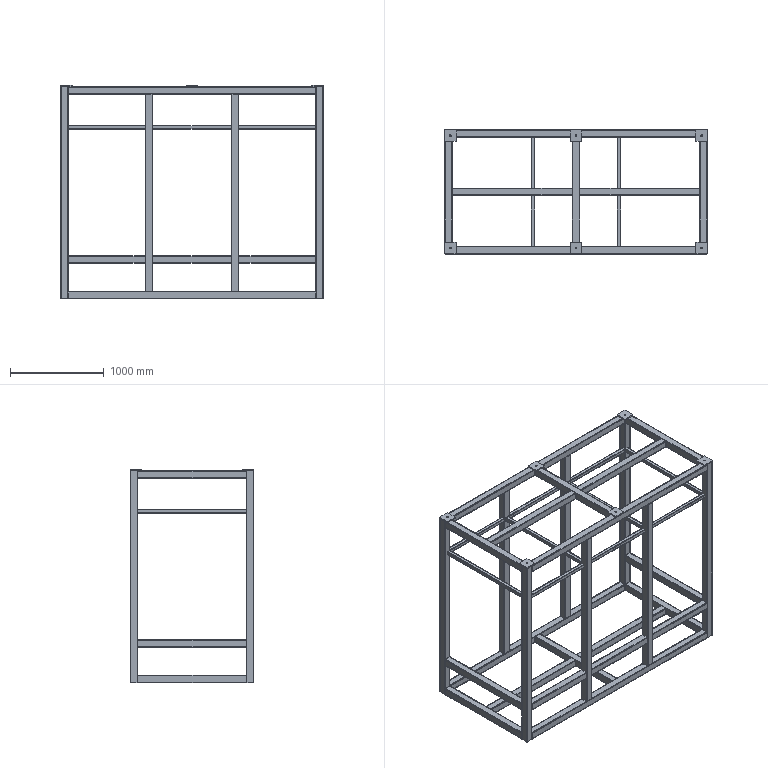Part | STEP file | Part4_default<as machined> | 43 solids | 718 faces | box 2800 x 1320 x 2280 mm | volume 47206904 mm3 | plane 406 | cylinder 312 | commonest cylinder face diameters 6.4 x108 12.8 x108 4 x40 8 x40 17.5 x16